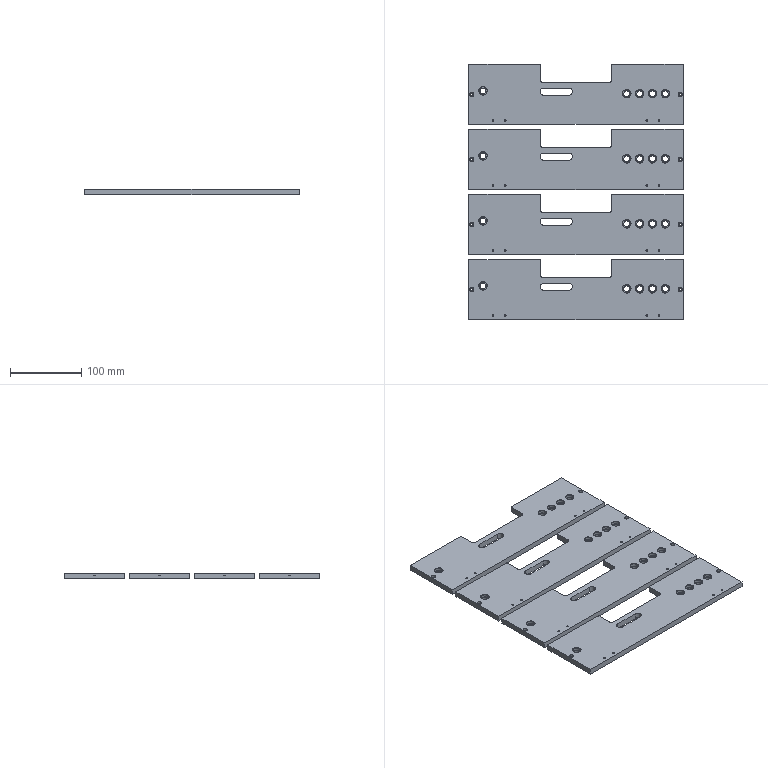Part | 4 solids | 316 faces | box 300 x 357 x 8 mm | volume 698910 mm3 | cylinder 184 | plane 76 | cone 56 | commonest cylinder face diameters 2.5 x48 8.1 x40 11 x40 3.5 x16 6 x16 2 x8